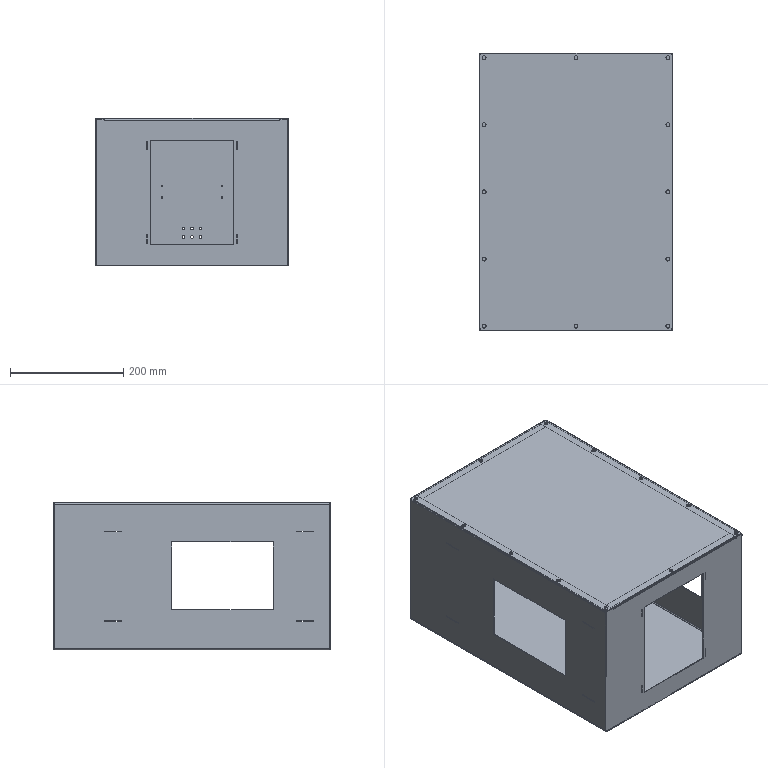Part | SolidWorks | 4 solids | 246 faces | box 340 x 490 x 261.2 mm | volume 851284 mm3 | plane 144 | cylinder 102 | commonest cylinder face diameters 7 x48 3 x18 5 x18 5.4 x14 10 x4